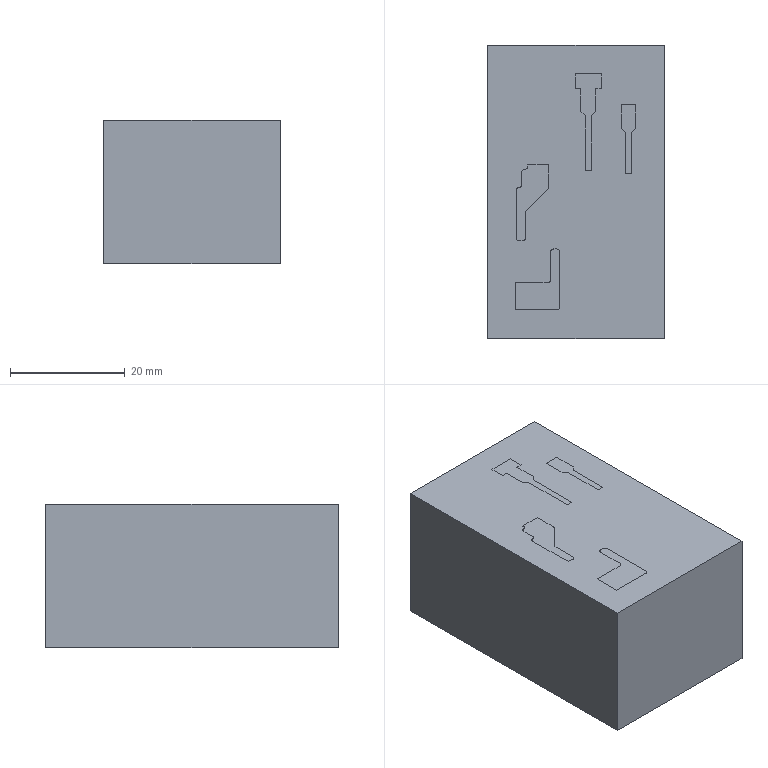Part | NX | features BREP 2 | 2 solids | 104 faces | box 30.723 x 50.978 x 25 mm | volume 71394 mm3 | plane 84 | cylinder 20 | commonest cylinder face diameters 1.1 x8 3.1 x8 0.9 x4